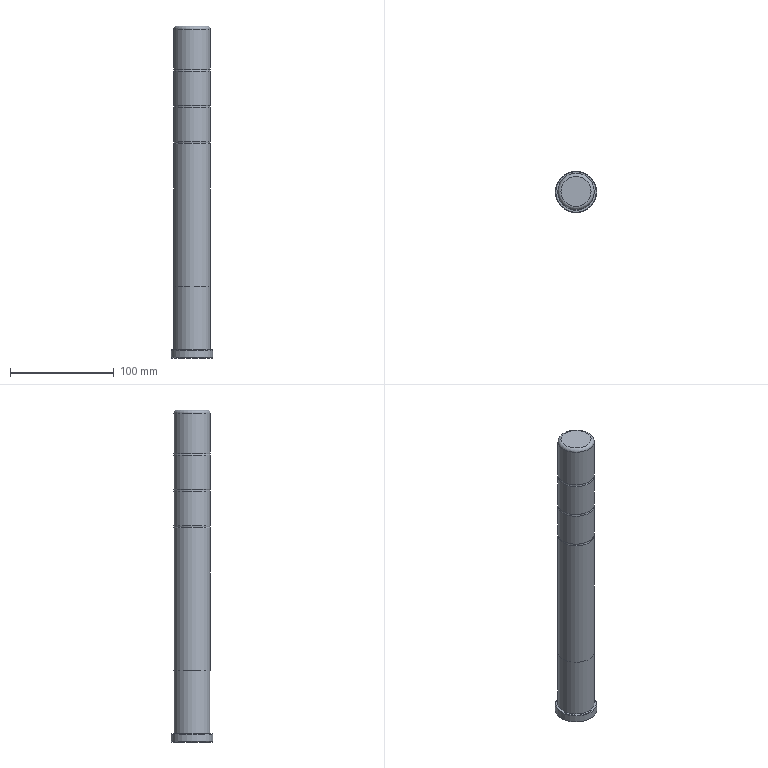Part | NX | features solid 2 | 1 solid | 16 faces | box 40 x 40 x 320 mm | volume 309816 mm3 | cylinder 6 | plane 4 | torus 4 | cone 2 | commonest cylinder face diameters 34.997 x4 35 x1 40 x1
STEP:
#1=CARTESIAN_POINT('',(179.5,-185.,-182.5));
#2=VERTEX_POINT('',#1);
#3=CARTESIAN_POINT('',(162.,-185.,-182.5));
#4=DIRECTION('',(0.,0.,1.));
#5=DIRECTION('',(1.,0.,0.));
#6=AXIS2_PLACEMENT_3D('',#3,#4,#5);
#7=CIRCLE('',#6,17.5);
#8=EDGE_CURVE('',#2,#2,#7,.T.);
#9=ORIENTED_EDGE('',*,*,#8,.F.);
#10=EDGE_LOOP('',(#9));
#11=FACE_BOUND('',#10,.T.);
#12=CARTESIAN_POINT('',(181.5,-185.,-182.5));
#13=VERTEX_POINT('',#12);
#14=CARTESIAN_POINT('',(162.,-185.,-182.5));
#15=DIRECTION('',(0.,0.,1.));
#16=DIRECTION('',(1.,0.,0.));
#17=AXIS2_PLACEMENT_3D('',#14,#15,#16);
#18=CIRCLE('',#17,19.5);
#19=EDGE_CURVE('',#13,#13,#18,.T.);
#20=ORIENTED_EDGE('',*,*,#19,.T.);
#21=EDGE_LOOP('',(#20));
#22=FACE_BOUND('',#21,.T.);
#23=CARTESIAN_POINT('',(162.,-185.,-182.5));
#24=DIRECTION('',(0.,0.,1.));
#25=DIRECTION('',(1.,0.,0.));
#26=AXIS2_PLACEMENT_3D('',#23,#24,#25);
#27=PLANE('',#26);
#28=ADVANCED_FACE('',(#11,#22),#27,.T.);
#29=CARTESIAN_POINT('',(142.5,-185.,-190.5));
#30=VERTEX_POINT('',#29);
#31=CARTESIAN_POINT('',(162.,-185.,-190.5));
#32=DIRECTION('',(0.,0.,-1.));
#33=DIRECTION('',(-1.,0.,0.));
#34=AXIS2_PLACEMENT_3D('',#31,#32,#33);
#35=CIRCLE('',#34,19.5);
#36=EDGE_CURVE('',#30,#30,#35,.T.);
#37=ORIENTED_EDGE('',*,*,#36,.T.);
#38=EDGE_LOOP('',(#37));
#39=FACE_BOUND('',#38,.T.);
#40=CARTESIAN_POINT('',(162.,-185.,-190.5));
#41=DIRECTION('',(0.,0.,-1.));
#42=DIRECTION('',(-1.,0.,0.));
#43=AXIS2_PLACEMENT_3D('',#40,#41,#42);
#44=PLANE('',#43);
#45=ADVANCED_FACE('',(#39),#44,.T.);
#46=CARTESIAN_POINT('',(142.,-185.,-190.));
#47=VERTEX_POINT('',#46);
#48=CARTESIAN_POINT('',(162.,-185.,-190.));
#49=DIRECTION('',(0.,0.,-1.));
#50=DIRECTION('',(-1.,0.,0.));
#51=AXIS2_PLACEMENT_3D('',#48,#49,#50);
#52=CIRCLE('',#51,20.);
#53=EDGE_CURVE('',#47,#47,#52,.F.);
#54=ORIENTED_EDGE('',*,*,#53,.T.);
#55=EDGE_LOOP('',(#54));
#56=FACE_BOUND('',#55,.T.);
#57=CARTESIAN_POINT('',(182.,-185.,-183.));
#58=VERTEX_POINT('',#57);
#59=CARTESIAN_POINT('',(162.,-185.,-183.));
#60=DIRECTION('',(0.,0.,1.));
#61=DIRECTION('',(1.,0.,0.));
#62=AXIS2_PLACEMENT_3D('',#59,#60,#61);
#63=CIRCLE('',#62,20.);
#64=EDGE_CURVE('',#58,#58,#63,.F.);
#65=ORIENTED_EDGE('',*,*,#64,.T.);
#66=EDGE_LOOP('',(#65));
#67=FACE_BOUND('',#66,.T.);
#68=CARTESIAN_POINT('',(162.,-185.,-190.5));
#69=DIRECTION('',(0.,0.,1.));
#70=DIRECTION('',(1.,0.,0.));
#71=AXIS2_PLACEMENT_3D('',#68,#69,#70);
#72=CYLINDRICAL_SURFACE('',#71,20.);
#73=ADVANCED_FACE('',(#56,#67),#72,.T.);
#74=ORIENTED_EDGE('',*,*,#36,.F.);
#75=EDGE_LOOP('',(#74));
#76=FACE_BOUND('',#75,.T.);
#77=ORIENTED_EDGE('',*,*,#53,.F.);
#78=EDGE_LOOP('',(#77));
#79=FACE_BOUND('',#78,.T.);
#80=CARTESIAN_POINT('',(162.,-185.,-190.));
#81=DIRECTION('',(0.,0.,1.));
#82=DIRECTION('',(1.,0.,0.));
#83=AXIS2_PLACEMENT_3D('',#80,#81,#82);
#84=CONICAL_SURFACE('',#83,20.,0.7854);
#85=ADVANCED_FACE('',(#76,#79),#84,.T.);
#86=ORIENTED_EDGE('',*,*,#19,.F.);
#87=EDGE_LOOP('',(#86));
#88=FACE_BOUND('',#87,.T.);
#89=ORIENTED_EDGE('',*,*,#64,.F.);
#90=EDGE_LOOP('',(#89));
#91=FACE_BOUND('',#90,.T.);
#92=CARTESIAN_POINT('',(162.,-185.,-183.));
#93=DIRECTION('',(0.,0.,-1.));
#94=DIRECTION('',(-1.,0.,0.));
#95=AXIS2_PLACEMENT_3D('',#92,#93,#94);
#96=CONICAL_SURFACE('',#95,20.,0.7854);
#97=ADVANCED_FACE('',(#88,#91),#96,.T.);
#98=CARTESIAN_POINT('',(179.499,-185.,-121.5));
#99=VERTEX_POINT('',#98);
#100=CARTESIAN_POINT('',(162.,-185.,-121.5));
#101=DIRECTION('',(0.,0.,1.));
#102=DIRECTION('',(1.,0.,0.));
#103=AXIS2_PLACEMENT_3D('',#100,#101,#102);
#104=CIRCLE('',#103,17.498);
#105=EDGE_CURVE('',#99,#99,#104,.T.);
#106=ORIENTED_EDGE('',*,*,#105,.F.);
#107=EDGE_LOOP('',(#106));
#108=FACE_BOUND('',#107,.T.);
#109=CARTESIAN_POINT('',(179.5,-185.,-121.5));
#110=VERTEX_POINT('',#109);
#111=CARTESIAN_POINT('',(162.,-185.,-121.5));
#112=DIRECTION('',(0.,0.,-1.));
#113=DIRECTION('',(1.,0.,0.));
#114=AXIS2_PLACEMENT_3D('',#111,#112,#113);
#115=CIRCLE('',#114,17.5);
#116=EDGE_CURVE('',#110,#110,#115,.T.);
#117=ORIENTED_EDGE('',*,*,#116,.F.);
#118=EDGE_LOOP('',(#117));
#119=FACE_BOUND('',#118,.T.);
#120=CARTESIAN_POINT('',(162.,-185.,-121.5));
#121=DIRECTION('',(0.,0.,1.));
#122=DIRECTION('',(1.,0.,0.));
#123=AXIS2_PLACEMENT_3D('',#120,#121,#122);
#124=PLANE('',#123);
#125=ADVANCED_FACE('',(#108,#119),#124,.T.);
#126=ORIENTED_EDGE('',*,*,#8,.T.);
#127=EDGE_LOOP('',(#126));
#128=FACE_BOUND('',#127,.T.);
#129=ORIENTED_EDGE('',*,*,#116,.T.);
#130=EDGE_LOOP('',(#129));
#131=FACE_BOUND('',#130,.T.);
#132=CARTESIAN_POINT('',(162.,-185.,-190.5));
#133=DIRECTION('',(0.,0.,1.));
#134=DIRECTION('',(1.,0.,0.));
#135=AXIS2_PLACEMENT_3D('',#132,#133,#134);
#136=CYLINDRICAL_SURFACE('',#135,17.5);
#137=ADVANCED_FACE('',(#128,#131),#136,.T.);
#138=CARTESIAN_POINT('',(179.499,-185.,15.949));
#139=VERTEX_POINT('',#138);
#140=CARTESIAN_POINT('',(162.,-185.,15.949));
#141=DIRECTION('',(0.,0.,1.));
#142=DIRECTION('',(1.,0.,0.));
#143=AXIS2_PLACEMENT_3D('',#140,#141,#142);
#144=CIRCLE('',#143,17.498);
#145=EDGE_CURVE('',#139,#139,#144,.T.);
#146=ORIENTED_EDGE('',*,*,#145,.F.);
#147=EDGE_LOOP('',(#146));
#148=FACE_BOUND('',#147,.T.);
#149=ORIENTED_EDGE('',*,*,#105,.T.);
#150=EDGE_LOOP('',(#149));
#151=FACE_BOUND('',#150,.T.);
#152=CARTESIAN_POINT('',(162.,-185.,-190.5));
#153=DIRECTION('',(0.,0.,1.));
#154=DIRECTION('',(1.,0.,0.));
#155=AXIS2_PLACEMENT_3D('',#152,#153,#154);
#156=CYLINDRICAL_SURFACE('',#155,17.498);
#157=ADVANCED_FACE('',(#148,#151),#156,.T.);
#158=CARTESIAN_POINT('',(144.501,-185.,18.051));
#159=VERTEX_POINT('',#158);
#160=CARTESIAN_POINT('',(162.,-185.,18.051));
#161=DIRECTION('',(0.,0.,-1.));
#162=DIRECTION('',(-1.,0.,0.));
#163=AXIS2_PLACEMENT_3D('',#160,#161,#162);
#164=CIRCLE('',#163,17.498);
#165=EDGE_CURVE('',#159,#159,#164,.T.);
#166=ORIENTED_EDGE('',*,*,#165,.T.);
#167=EDGE_LOOP('',(#166));
#168=FACE_BOUND('',#167,.T.);
#169=ORIENTED_EDGE('',*,*,#145,.T.);
#170=EDGE_LOOP('',(#169));
#171=FACE_BOUND('',#170,.T.);
#172=CARTESIAN_POINT('',(162.,-185.,17.));
#173=DIRECTION('',(0.,0.,1.));
#174=DIRECTION('',(1.,0.,0.));
#175=AXIS2_PLACEMENT_3D('',#172,#173,#174);
#176=TOROIDAL_SURFACE('',#175,19.2,2.);
#177=ADVANCED_FACE('',(#168,#171),#176,.F.);
#178=CARTESIAN_POINT('',(179.499,-185.,50.949));
#179=VERTEX_POINT('',#178);
#180=CARTESIAN_POINT('',(162.,-185.,50.949));
#181=DIRECTION('',(0.,0.,1.));
#182=DIRECTION('',(1.,0.,0.));
#183=AXIS2_PLACEMENT_3D('',#180,#181,#182);
#184=CIRCLE('',#183,17.498);
#185=EDGE_CURVE('',#179,#179,#184,.T.);
#186=ORIENTED_EDGE('',*,*,#185,.F.);
#187=EDGE_LOOP('',(#186));
#188=FACE_BOUND('',#187,.T.);
#189=ORIENTED_EDGE('',*,*,#165,.F.);
#190=EDGE_LOOP('',(#189));
#191=FACE_BOUND('',#190,.T.);
#192=CARTESIAN_POINT('',(162.,-185.,-190.5));
#193=DIRECTION('',(0.,0.,1.));
#194=DIRECTION('',(1.,0.,0.));
#195=AXIS2_PLACEMENT_3D('',#192,#193,#194);
#196=CYLINDRICAL_SURFACE('',#195,17.498);
#197=ADVANCED_FACE('',(#188,#191),#196,.T.);
#198=CARTESIAN_POINT('',(144.501,-185.,53.051));
#199=VERTEX_POINT('',#198);
#200=CARTESIAN_POINT('',(162.,-185.,53.051));
#201=DIRECTION('',(0.,0.,-1.));
#202=DIRECTION('',(-1.,0.,0.));
#203=AXIS2_PLACEMENT_3D('',#200,#201,#202);
#204=CIRCLE('',#203,17.498);
#205=EDGE_CURVE('',#199,#199,#204,.T.);
#206=ORIENTED_EDGE('',*,*,#205,.T.);
#207=EDGE_LOOP('',(#206));
#208=FACE_BOUND('',#207,.T.);
#209=ORIENTED_EDGE('',*,*,#185,.T.);
#210=EDGE_LOOP('',(#209));
#211=FACE_BOUND('',#210,.T.);
#212=CARTESIAN_POINT('',(162.,-185.,52.));
#213=DIRECTION('',(0.,0.,1.));
#214=DIRECTION('',(1.,0.,0.));
#215=AXIS2_PLACEMENT_3D('',#212,#213,#214);
#216=TOROIDAL_SURFACE('',#215,19.2,2.);
#217=ADVANCED_FACE('',(#208,#211),#216,.F.);
#218=CARTESIAN_POINT('',(179.499,-185.,85.949));
#219=VERTEX_POINT('',#218);
#220=CARTESIAN_POINT('',(162.,-185.,85.949));
#221=DIRECTION('',(0.,0.,1.));
#222=DIRECTION('',(1.,0.,0.));
#223=AXIS2_PLACEMENT_3D('',#220,#221,#222);
#224=CIRCLE('',#223,17.498);
#225=EDGE_CURVE('',#219,#219,#224,.T.);
#226=ORIENTED_EDGE('',*,*,#225,.F.);
#227=EDGE_LOOP('',(#226));
#228=FACE_BOUND('',#227,.T.);
#229=ORIENTED_EDGE('',*,*,#205,.F.);
#230=EDGE_LOOP('',(#229));
#231=FACE_BOUND('',#230,.T.);
#232=CARTESIAN_POINT('',(162.,-185.,-190.5));
#233=DIRECTION('',(0.,0.,1.));
#234=DIRECTION('',(1.,0.,0.));
#235=AXIS2_PLACEMENT_3D('',#232,#233,#234);
#236=CYLINDRICAL_SURFACE('',#235,17.498);
#237=ADVANCED_FACE('',(#228,#231),#236,.T.);
#238=CARTESIAN_POINT('',(144.501,-185.,88.051));
#239=VERTEX_POINT('',#238);
#240=CARTESIAN_POINT('',(162.,-185.,88.051));
#241=DIRECTION('',(0.,0.,-1.));
#242=DIRECTION('',(-1.,0.,0.));
#243=AXIS2_PLACEMENT_3D('',#240,#241,#242);
#244=CIRCLE('',#243,17.498);
#245=EDGE_CURVE('',#239,#239,#244,.T.);
#246=ORIENTED_EDGE('',*,*,#245,.T.);
#247=EDGE_LOOP('',(#246));
#248=FACE_BOUND('',#247,.T.);
#249=ORIENTED_EDGE('',*,*,#225,.T.);
#250=EDGE_LOOP('',(#249));
#251=FACE_BOUND('',#250,.T.);
#252=CARTESIAN_POINT('',(162.,-185.,87.));
#253=DIRECTION('',(0.,0.,1.));
#254=DIRECTION('',(1.,0.,0.));
#255=AXIS2_PLACEMENT_3D('',#252,#253,#254);
#256=TOROIDAL_SURFACE('',#255,19.2,2.);
#257=ADVANCED_FACE('',(#248,#251),#256,.F.);
#258=CARTESIAN_POINT('',(176.499,-185.,129.5));
#259=VERTEX_POINT('',#258);
#260=CARTESIAN_POINT('',(162.,-185.,129.5));
#261=DIRECTION('',(0.,0.,1.));
#262=DIRECTION('',(1.,0.,0.));
#263=AXIS2_PLACEMENT_3D('',#260,#261,#262);
#264=CIRCLE('',#263,14.498);
#265=EDGE_CURVE('',#259,#259,#264,.T.);
#266=ORIENTED_EDGE('',*,*,#265,.T.);
#267=EDGE_LOOP('',(#266));
#268=FACE_BOUND('',#267,.T.);
#269=CARTESIAN_POINT('',(162.,-185.,129.5));
#270=DIRECTION('',(0.,0.,1.));
#271=DIRECTION('',(1.,0.,0.));
#272=AXIS2_PLACEMENT_3D('',#269,#270,#271);
#273=PLANE('',#272);
#274=ADVANCED_FACE('',(#268),#273,.T.);
#275=ORIENTED_EDGE('',*,*,#265,.F.);
#276=EDGE_LOOP('',(#275));
#277=FACE_BOUND('',#276,.T.);
#278=CARTESIAN_POINT('',(179.499,-185.,126.5));
#279=VERTEX_POINT('',#278);
#280=CARTESIAN_POINT('',(162.,-185.,126.5));
#281=DIRECTION('',(0.,0.,1.));
#282=DIRECTION('',(1.,0.,0.));
#283=AXIS2_PLACEMENT_3D('',#280,#281,#282);
#284=CIRCLE('',#283,17.498);
#285=EDGE_CURVE('',#279,#279,#284,.F.);
#286=ORIENTED_EDGE('',*,*,#285,.F.);
#287=EDGE_LOOP('',(#286));
#288=FACE_BOUND('',#287,.T.);
#289=CARTESIAN_POINT('',(162.,-185.,126.5));
#290=DIRECTION('',(0.,0.,1.));
#291=DIRECTION('',(1.,0.,0.));
#292=AXIS2_PLACEMENT_3D('',#289,#290,#291);
#293=TOROIDAL_SURFACE('',#292,14.498,3.);
#294=ADVANCED_FACE('',(#277,#288),#293,.T.);
#295=ORIENTED_EDGE('',*,*,#245,.F.);
#296=EDGE_LOOP('',(#295));
#297=FACE_BOUND('',#296,.T.);
#298=ORIENTED_EDGE('',*,*,#285,.T.);
#299=EDGE_LOOP('',(#298));
#300=FACE_BOUND('',#299,.T.);
#301=CARTESIAN_POINT('',(162.,-185.,-190.5));
#302=DIRECTION('',(0.,0.,1.));
#303=DIRECTION('',(1.,0.,0.));
#304=AXIS2_PLACEMENT_3D('',#301,#302,#303);
#305=CYLINDRICAL_SURFACE('',#304,17.498);
#306=ADVANCED_FACE('',(#297,#300),#305,.T.);
#307=CLOSED_SHELL('',(#28,#45,#73,#85,#97,#125,#137,#157,#177,#197,#217,#237,#257,#274,#294,#306));
#308=MANIFOLD_SOLID_BREP('',#307);
#309=(LENGTH_UNIT()NAMED_UNIT(*)SI_UNIT(.MILLI.,.METRE.));
#310=UNCERTAINTY_MEASURE_WITH_UNIT(LENGTH_MEASURE(0.00001),#309,'','');
#311=(NAMED_UNIT(*)PLANE_ANGLE_UNIT()SI_UNIT($,.RADIAN.));
#312=(NAMED_UNIT(*)SI_UNIT($,.STERADIAN.)SOLID_ANGLE_UNIT());
#313=(GEOMETRIC_REPRESENTATION_CONTEXT(3)GLOBAL_UNCERTAINTY_ASSIGNED_CONTEXT((#310))GLOBAL_UNIT_ASSIGNED_CONTEXT((#309,#311,#312))REPRESENTATION_CONTEXT('',''));
#314=ADVANCED_BREP_SHAPE_REPRESENTATION('',(#308),#313);